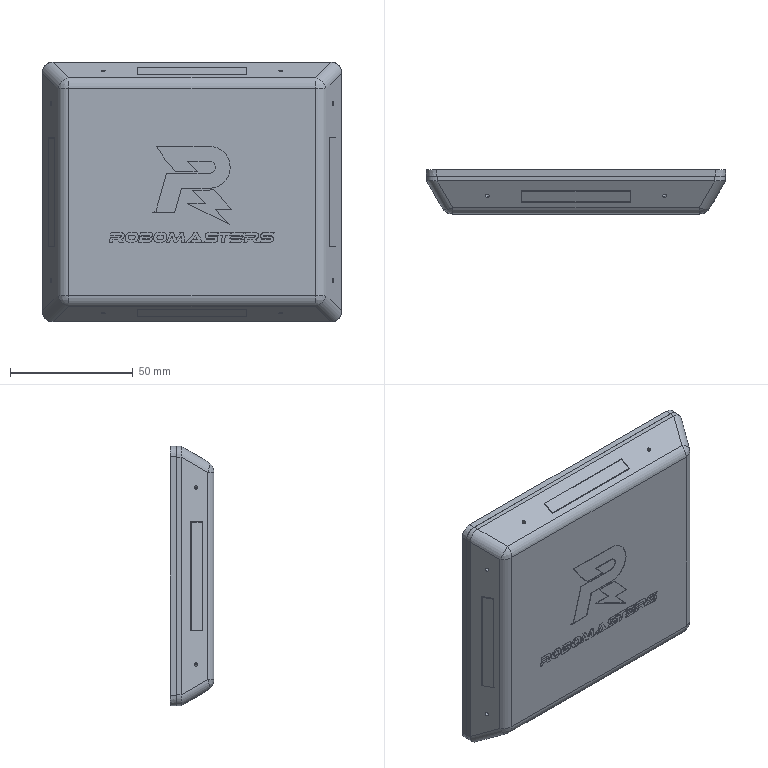Part | SolidWorks | features BaseBody 6 | 6 solids | 564 faces | box 121.675 x 17.8 x 105.675 mm | volume 74088 mm3 | plane 277 | spline 143 | cylinder 76 | cone 64 | sphere 4 | commonest cylinder face diameters 1.5 x16 2 x16 3 x8 3.2 x8 4 x8 4.5 x8